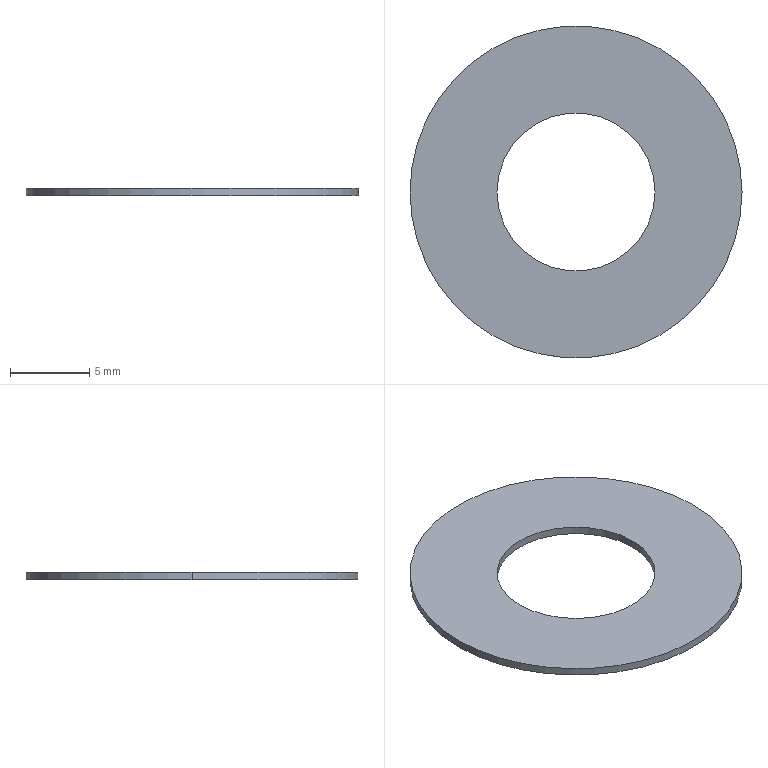Part | SolidWorks | features Extrusion 1 | 1 solid | 6 faces | box 21 x 21 x 0.5 mm | volume 133.91 mm3 | cylinder 4 | plane 2 | commonest cylinder face diameters 10 x2 21 x2
STEP:
#1=CARTESIAN_POINT('',(-126.531,115.619,0.5));
#2=VERTEX_POINT('',#1);
#3=CARTESIAN_POINT('',(-116.531,115.619,0.5));
#4=VERTEX_POINT('',#3);
#5=CARTESIAN_POINT('',(-121.531,115.619,0.5));
#6=DIRECTION('',(0.,0.,1.));
#7=DIRECTION('',(1.,0.,0.));
#8=AXIS2_PLACEMENT_3D('',#5,#6,#7);
#9=CIRCLE('',#8,5.);
#10=EDGE_CURVE('',#2,#4,#9,.T.);
#11=ORIENTED_EDGE('',*,*,#10,.T.);
#12=CARTESIAN_POINT('',(-116.531,115.619,0.));
#13=VERTEX_POINT('',#12);
#14=CARTESIAN_POINT('',(-116.531,115.619,0.5));
#15=DIRECTION('',(0.,0.,-1.));
#16=VECTOR('',#15,1000.);
#17=LINE('',#14,#16);
#18=EDGE_CURVE('',#4,#13,#17,.T.);
#19=ORIENTED_EDGE('',*,*,#18,.T.);
#20=CARTESIAN_POINT('',(-126.531,115.619,0.));
#21=VERTEX_POINT('',#20);
#22=CARTESIAN_POINT('',(-121.531,115.619,0.));
#23=DIRECTION('',(0.,0.,1.));
#24=DIRECTION('',(1.,0.,0.));
#25=AXIS2_PLACEMENT_3D('',#22,#23,#24);
#26=CIRCLE('',#25,5.);
#27=EDGE_CURVE('',#21,#13,#26,.T.);
#28=ORIENTED_EDGE('',*,*,#27,.F.);
#29=CARTESIAN_POINT('',(-126.531,115.619,0.5));
#30=DIRECTION('',(0.,0.,-1.));
#31=VECTOR('',#30,1000.);
#32=LINE('',#29,#31);
#33=EDGE_CURVE('',#2,#21,#32,.T.);
#34=ORIENTED_EDGE('',*,*,#33,.F.);
#35=EDGE_LOOP('',(#11,#19,#28,#34));
#36=FACE_OUTER_BOUND('',#35,.T.);
#37=CARTESIAN_POINT('',(-121.531,115.619,0.5));
#38=DIRECTION('',(0.,0.,-1.));
#39=DIRECTION('',(-1.,0.,0.));
#40=AXIS2_PLACEMENT_3D('',#37,#38,#39);
#41=CYLINDRICAL_SURFACE('',#40,5.);
#42=ADVANCED_FACE('',(#36),#41,.F.);
#43=CARTESIAN_POINT('',(-111.031,115.619,0.5));
#44=VERTEX_POINT('',#43);
#45=CARTESIAN_POINT('',(-132.031,115.619,0.5));
#46=VERTEX_POINT('',#45);
#47=CARTESIAN_POINT('',(-121.531,115.619,0.5));
#48=DIRECTION('',(0.,0.,1.));
#49=DIRECTION('',(1.,0.,0.));
#50=AXIS2_PLACEMENT_3D('',#47,#48,#49);
#51=CIRCLE('',#50,10.5);
#52=EDGE_CURVE('',#44,#46,#51,.T.);
#53=ORIENTED_EDGE('',*,*,#52,.F.);
#54=CARTESIAN_POINT('',(-111.031,115.619,0.));
#55=VERTEX_POINT('',#54);
#56=CARTESIAN_POINT('',(-111.031,115.619,0.5));
#57=DIRECTION('',(0.,0.,-1.));
#58=VECTOR('',#57,1000.);
#59=LINE('',#56,#58);
#60=EDGE_CURVE('',#44,#55,#59,.T.);
#61=ORIENTED_EDGE('',*,*,#60,.T.);
#62=CARTESIAN_POINT('',(-132.031,115.619,0.));
#63=VERTEX_POINT('',#62);
#64=CARTESIAN_POINT('',(-121.531,115.619,0.));
#65=DIRECTION('',(0.,0.,1.));
#66=DIRECTION('',(1.,0.,0.));
#67=AXIS2_PLACEMENT_3D('',#64,#65,#66);
#68=CIRCLE('',#67,10.5);
#69=EDGE_CURVE('',#55,#63,#68,.T.);
#70=ORIENTED_EDGE('',*,*,#69,.T.);
#71=CARTESIAN_POINT('',(-132.031,115.619,0.5));
#72=DIRECTION('',(0.,0.,-1.));
#73=VECTOR('',#72,1000.);
#74=LINE('',#71,#73);
#75=EDGE_CURVE('',#46,#63,#74,.T.);
#76=ORIENTED_EDGE('',*,*,#75,.F.);
#77=EDGE_LOOP('',(#53,#61,#70,#76));
#78=FACE_OUTER_BOUND('',#77,.T.);
#79=CARTESIAN_POINT('',(-121.531,115.619,0.5));
#80=DIRECTION('',(0.,0.,-1.));
#81=DIRECTION('',(-1.,0.,0.));
#82=AXIS2_PLACEMENT_3D('',#79,#80,#81);
#83=CYLINDRICAL_SURFACE('',#82,10.5);
#84=ADVANCED_FACE('',(#78),#83,.T.);
#85=CARTESIAN_POINT('',(-121.531,115.619,0.5));
#86=DIRECTION('',(0.,0.,1.));
#87=DIRECTION('',(1.,0.,0.));
#88=AXIS2_PLACEMENT_3D('',#85,#86,#87);
#89=CIRCLE('',#88,10.5);
#90=EDGE_CURVE('',#46,#44,#89,.T.);
#91=ORIENTED_EDGE('',*,*,#90,.T.);
#92=ORIENTED_EDGE('',*,*,#52,.T.);
#93=EDGE_LOOP('',(#91,#92));
#94=FACE_OUTER_BOUND('',#93,.T.);
#95=ORIENTED_EDGE('',*,*,#10,.F.);
#96=CARTESIAN_POINT('',(-121.531,115.619,0.5));
#97=DIRECTION('',(0.,0.,1.));
#98=DIRECTION('',(1.,0.,0.));
#99=AXIS2_PLACEMENT_3D('',#96,#97,#98);
#100=CIRCLE('',#99,5.);
#101=EDGE_CURVE('',#4,#2,#100,.T.);
#102=ORIENTED_EDGE('',*,*,#101,.F.);
#103=EDGE_LOOP('',(#95,#102));
#104=FACE_BOUND('',#103,.T.);
#105=CARTESIAN_POINT('',(-121.531,115.619,0.5));
#106=DIRECTION('',(0.,0.,1.));
#107=DIRECTION('',(1.,0.,0.));
#108=AXIS2_PLACEMENT_3D('',#105,#106,#107);
#109=PLANE('',#108);
#110=ADVANCED_FACE('',(#94,#104),#109,.T.);
#111=CARTESIAN_POINT('',(-121.531,115.619,0.));
#112=DIRECTION('',(0.,0.,1.));
#113=DIRECTION('',(1.,0.,0.));
#114=AXIS2_PLACEMENT_3D('',#111,#112,#113);
#115=CIRCLE('',#114,10.5);
#116=EDGE_CURVE('',#63,#55,#115,.T.);
#117=ORIENTED_EDGE('',*,*,#116,.F.);
#118=ORIENTED_EDGE('',*,*,#69,.F.);
#119=EDGE_LOOP('',(#117,#118));
#120=FACE_OUTER_BOUND('',#119,.T.);
#121=ORIENTED_EDGE('',*,*,#27,.T.);
#122=CARTESIAN_POINT('',(-121.531,115.619,0.));
#123=DIRECTION('',(0.,0.,1.));
#124=DIRECTION('',(1.,0.,0.));
#125=AXIS2_PLACEMENT_3D('',#122,#123,#124);
#126=CIRCLE('',#125,5.);
#127=EDGE_CURVE('',#13,#21,#126,.T.);
#128=ORIENTED_EDGE('',*,*,#127,.T.);
#129=EDGE_LOOP('',(#121,#128));
#130=FACE_BOUND('',#129,.T.);
#131=CARTESIAN_POINT('',(-121.531,115.619,0.));
#132=DIRECTION('',(0.,0.,1.));
#133=DIRECTION('',(1.,0.,0.));
#134=AXIS2_PLACEMENT_3D('',#131,#132,#133);
#135=PLANE('',#134);
#136=ADVANCED_FACE('',(#120,#130),#135,.F.);
#137=ORIENTED_EDGE('',*,*,#60,.F.);
#138=ORIENTED_EDGE('',*,*,#90,.F.);
#139=ORIENTED_EDGE('',*,*,#75,.T.);
#140=ORIENTED_EDGE('',*,*,#116,.T.);
#141=EDGE_LOOP('',(#137,#138,#139,#140));
#142=FACE_OUTER_BOUND('',#141,.T.);
#143=CARTESIAN_POINT('',(-121.531,115.619,0.5));
#144=DIRECTION('',(0.,0.,-1.));
#145=DIRECTION('',(-1.,0.,0.));
#146=AXIS2_PLACEMENT_3D('',#143,#144,#145);
#147=CYLINDRICAL_SURFACE('',#146,10.5);
#148=ADVANCED_FACE('',(#142),#147,.T.);
#149=ORIENTED_EDGE('',*,*,#18,.F.);
#150=ORIENTED_EDGE('',*,*,#101,.T.);
#151=ORIENTED_EDGE('',*,*,#33,.T.);
#152=ORIENTED_EDGE('',*,*,#127,.F.);
#153=EDGE_LOOP('',(#149,#150,#151,#152));
#154=FACE_OUTER_BOUND('',#153,.T.);
#155=CARTESIAN_POINT('',(-121.531,115.619,0.5));
#156=DIRECTION('',(0.,0.,-1.));
#157=DIRECTION('',(-1.,0.,0.));
#158=AXIS2_PLACEMENT_3D('',#155,#156,#157);
#159=CYLINDRICAL_SURFACE('',#158,5.);
#160=ADVANCED_FACE('',(#154),#159,.F.);
#161=CLOSED_SHELL('',(#42,#84,#110,#136,#148,#160));
#162=MANIFOLD_SOLID_BREP('',#161);
#163=CARTESIAN_POINT('',(0.,0.,0.));
#164=DIRECTION('',(0.,0.,1.));
#165=DIRECTION('',(1.,0.,0.));
#166=AXIS2_PLACEMENT_3D('',#163,#164,#165);
#167=(LENGTH_UNIT()NAMED_UNIT(*)SI_UNIT(.MILLI.,.METRE.));
#168=UNCERTAINTY_MEASURE_WITH_UNIT(LENGTH_MEASURE(0.00001),#167,'','');
#169=(NAMED_UNIT(*)PLANE_ANGLE_UNIT()SI_UNIT($,.RADIAN.));
#170=(NAMED_UNIT(*)SI_UNIT($,.STERADIAN.)SOLID_ANGLE_UNIT());
#171=(GEOMETRIC_REPRESENTATION_CONTEXT(3)GLOBAL_UNCERTAINTY_ASSIGNED_CONTEXT((#168))GLOBAL_UNIT_ASSIGNED_CONTEXT((#167,#169,#170))REPRESENTATION_CONTEXT('',''));
#172=ADVANCED_BREP_SHAPE_REPRESENTATION('',(#162,#166),#171);